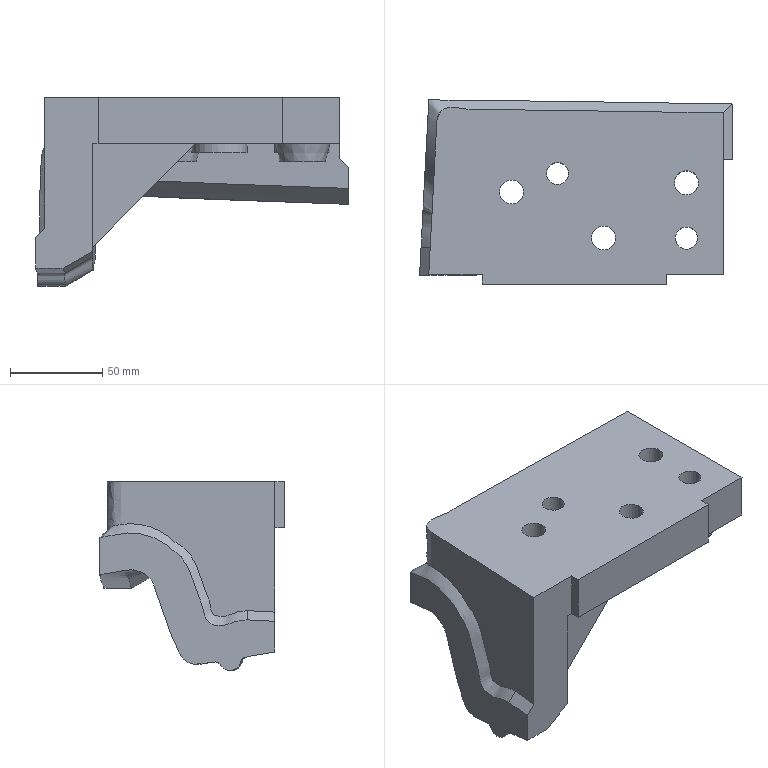Part | NX | features solid 2 | 1 solid | 45 faces | box 170.219 x 100.132 x 102.654 mm | volume 621282 mm3 | plane 24 | cylinder 11 | spline 8 | cone 2 | commonest cylinder face diameters 13 x5 12 x2 30 x2 32 x2